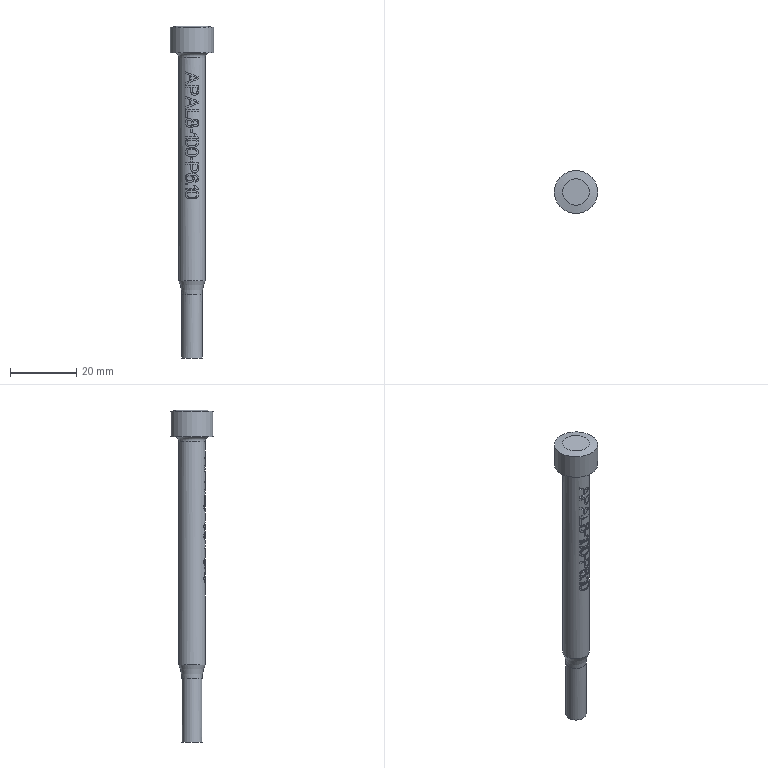Part | STEP file | PN_0049_id1058_x_t | 1 solid | 186 faces | box 13 x 13 x 100 mm | volume 5213 mm3 | plane 106 | cylinder 77 | torus 2 | cone 1 | commonest cylinder face diameters 7.8 x15 8 x11 1.671 x3 1.994 x3 2 x3 2.024 x3